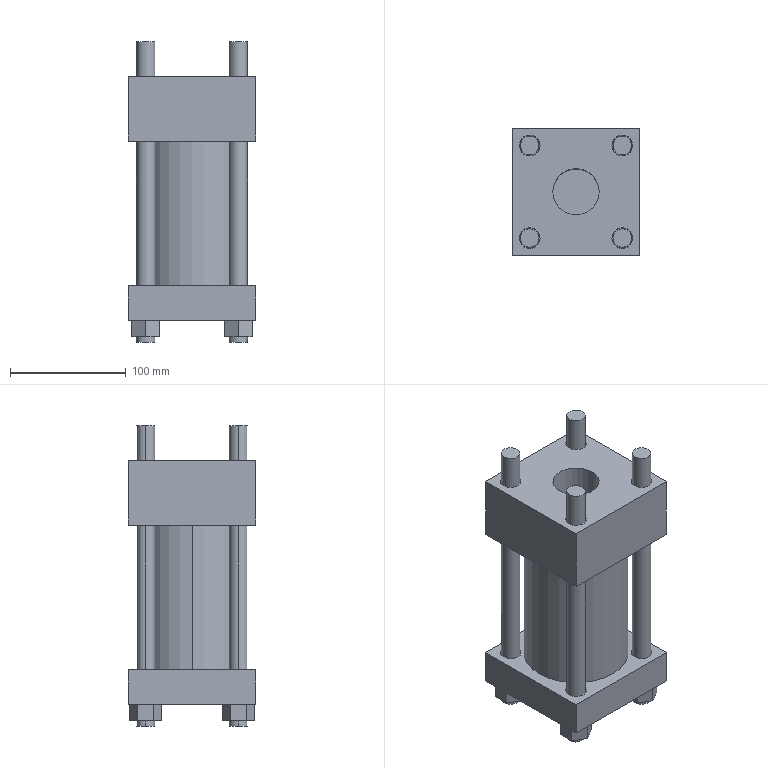Part | STEP file | XYLANH _S_^80 | 1 solid | 95 faces | box 110 x 110 x 260 mm | volume 1251491 mm3 | plane 55 | cylinder 40 | commonest cylinder face diameters 16 x16 18 x16 40 x4 80 x2 90 x2